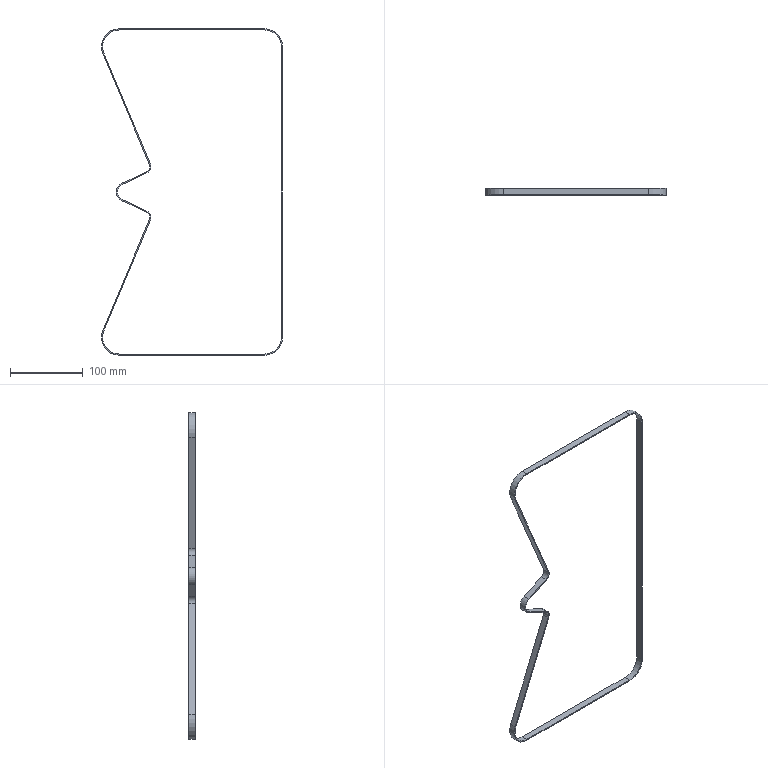Part | SolidWorks | features Extrusion 1 | 1 solid | 30 faces | box 248.84 x 9 x 448.84 mm | volume 19272 mm3 | plane 16 | cylinder 14 | commonest cylinder face diameters 45.84 x4 48.84 x4 16 x2 19 x2 22.92 x1 25.92 x1
STEP:
#1=CARTESIAN_POINT('',(121.194,9.,924.42));
#2=VERTEX_POINT('',#1);
#3=CARTESIAN_POINT('',(145.614,9.,900.));
#4=VERTEX_POINT('',#3);
#5=CARTESIAN_POINT('',(121.194,9.,900.));
#6=DIRECTION('',(0.,1.,0.));
#7=DIRECTION('',(0.,0.,1.));
#8=AXIS2_PLACEMENT_3D('',#5,#6,#7);
#9=CIRCLE('',#8,24.42);
#10=EDGE_CURVE('',#2,#4,#9,.T.);
#11=ORIENTED_EDGE('',*,*,#10,.T.);
#12=CARTESIAN_POINT('',(145.614,9.,500.));
#13=VERTEX_POINT('',#12);
#14=CARTESIAN_POINT('',(145.614,9.,900.));
#15=DIRECTION('',(0.,0.,-1.));
#16=VECTOR('',#15,1000.);
#17=LINE('',#14,#16);
#18=EDGE_CURVE('',#4,#13,#17,.T.);
#19=ORIENTED_EDGE('',*,*,#18,.T.);
#20=CARTESIAN_POINT('',(121.194,9.,475.58));
#21=VERTEX_POINT('',#20);
#22=CARTESIAN_POINT('',(121.194,9.,500.));
#23=DIRECTION('',(0.,1.,0.));
#24=DIRECTION('',(0.,0.,1.));
#25=AXIS2_PLACEMENT_3D('',#22,#23,#24);
#26=CIRCLE('',#25,24.42);
#27=EDGE_CURVE('',#13,#21,#26,.T.);
#28=ORIENTED_EDGE('',*,*,#27,.T.);
#29=CARTESIAN_POINT('',(-78.806,9.,475.58));
#30=VERTEX_POINT('',#29);
#31=CARTESIAN_POINT('',(121.194,9.,475.58));
#32=DIRECTION('',(-1.,0.,0.));
#33=VECTOR('',#32,1000.);
#34=LINE('',#31,#33);
#35=EDGE_CURVE('',#21,#30,#34,.T.);
#36=ORIENTED_EDGE('',*,*,#35,.T.);
#37=CARTESIAN_POINT('',(-101.328,9.,509.439));
#38=VERTEX_POINT('',#37);
#39=CARTESIAN_POINT('',(-78.806,9.,500.));
#40=DIRECTION('',(0.,1.,0.));
#41=DIRECTION('',(0.,0.,1.));
#42=AXIS2_PLACEMENT_3D('',#39,#40,#41);
#43=CIRCLE('',#42,24.42);
#44=EDGE_CURVE('',#30,#38,#43,.T.);
#45=ORIENTED_EDGE('',*,*,#44,.T.);
#46=CARTESIAN_POINT('',(-37.428,9.,661.908));
#47=VERTEX_POINT('',#46);
#48=CARTESIAN_POINT('',(-37.428,9.,661.908));
#49=DIRECTION('',(0.3865,0.,0.9223));
#50=VECTOR('',#49,1000.);
#51=LINE('',#48,#50);
#52=EDGE_CURVE('',#38,#47,#51,.T.);
#53=ORIENTED_EDGE('',*,*,#52,.T.);
#54=CARTESIAN_POINT('',(-41.387,9.,672.233));
#55=VERTEX_POINT('',#54);
#56=CARTESIAN_POINT('',(-44.806,9.,665.));
#57=DIRECTION('',(0.,-1.,0.));
#58=DIRECTION('',(0.,0.,1.));
#59=AXIS2_PLACEMENT_3D('',#56,#57,#58);
#60=CIRCLE('',#59,8.);
#61=EDGE_CURVE('',#47,#55,#60,.T.);
#62=ORIENTED_EDGE('',*,*,#61,.T.);
#63=CARTESIAN_POINT('',(-75.344,9.,688.283));
#64=VERTEX_POINT('',#63);
#65=CARTESIAN_POINT('',(-75.344,9.,688.283));
#66=DIRECTION('',(-0.9041,0.,0.4273));
#67=VECTOR('',#66,1000.);
#68=LINE('',#65,#67);
#69=EDGE_CURVE('',#55,#64,#68,.T.);
#70=ORIENTED_EDGE('',*,*,#69,.T.);
#71=CARTESIAN_POINT('',(-75.344,9.,711.717));
#72=VERTEX_POINT('',#71);
#73=CARTESIAN_POINT('',(-69.806,9.,700.));
#74=DIRECTION('',(0.,1.,0.));
#75=DIRECTION('',(0.,0.,1.));
#76=AXIS2_PLACEMENT_3D('',#73,#74,#75);
#77=CIRCLE('',#76,12.96);
#78=EDGE_CURVE('',#64,#72,#77,.T.);
#79=ORIENTED_EDGE('',*,*,#78,.T.);
#80=CARTESIAN_POINT('',(-41.387,9.,727.767));
#81=VERTEX_POINT('',#80);
#82=CARTESIAN_POINT('',(-75.344,9.,711.717));
#83=DIRECTION('',(0.9041,0.,0.4273));
#84=VECTOR('',#83,1000.);
#85=LINE('',#82,#84);
#86=EDGE_CURVE('',#72,#81,#85,.T.);
#87=ORIENTED_EDGE('',*,*,#86,.T.);
#88=CARTESIAN_POINT('',(-37.428,9.,738.092));
#89=VERTEX_POINT('',#88);
#90=CARTESIAN_POINT('',(-44.806,9.,735.));
#91=DIRECTION('',(0.,-1.,0.));
#92=DIRECTION('',(0.,0.,1.));
#93=AXIS2_PLACEMENT_3D('',#90,#91,#92);
#94=CIRCLE('',#93,8.);
#95=EDGE_CURVE('',#81,#89,#94,.T.);
#96=ORIENTED_EDGE('',*,*,#95,.T.);
#97=CARTESIAN_POINT('',(-101.328,9.,890.561));
#98=VERTEX_POINT('',#97);
#99=CARTESIAN_POINT('',(-37.428,9.,738.092));
#100=DIRECTION('',(-0.3865,0.,0.9223));
#101=VECTOR('',#100,1000.);
#102=LINE('',#99,#101);
#103=EDGE_CURVE('',#89,#98,#102,.T.);
#104=ORIENTED_EDGE('',*,*,#103,.T.);
#105=CARTESIAN_POINT('',(-78.806,9.,924.42));
#106=VERTEX_POINT('',#105);
#107=CARTESIAN_POINT('',(-78.806,9.,900.));
#108=DIRECTION('',(0.,1.,0.));
#109=DIRECTION('',(0.,0.,1.));
#110=AXIS2_PLACEMENT_3D('',#107,#108,#109);
#111=CIRCLE('',#110,24.42);
#112=EDGE_CURVE('',#98,#106,#111,.T.);
#113=ORIENTED_EDGE('',*,*,#112,.T.);
#114=CARTESIAN_POINT('',(121.194,9.,924.42));
#115=DIRECTION('',(1.,0.,0.));
#116=VECTOR('',#115,1000.);
#117=LINE('',#114,#116);
#118=EDGE_CURVE('',#106,#2,#117,.T.);
#119=ORIENTED_EDGE('',*,*,#118,.T.);
#120=EDGE_LOOP('',(#11,#19,#28,#36,#45,#53,#62,#70,#79,#87,#96,#104,#113,#119));
#121=FACE_OUTER_BOUND('',#120,.T.);
#122=CARTESIAN_POINT('',(-40.746,9.,673.589));
#123=VERTEX_POINT('',#122);
#124=CARTESIAN_POINT('',(-74.703,9.,689.639));
#125=VERTEX_POINT('',#124);
#126=CARTESIAN_POINT('',(-74.703,9.,689.639));
#127=DIRECTION('',(-0.9041,0.,0.4273));
#128=VECTOR('',#127,1000.);
#129=LINE('',#126,#128);
#130=EDGE_CURVE('',#123,#125,#129,.T.);
#131=ORIENTED_EDGE('',*,*,#130,.F.);
#132=CARTESIAN_POINT('',(-36.044,9.,661.328));
#133=VERTEX_POINT('',#132);
#134=CARTESIAN_POINT('',(-44.806,9.,665.));
#135=DIRECTION('',(0.,-1.,0.));
#136=DIRECTION('',(0.,0.,1.));
#137=AXIS2_PLACEMENT_3D('',#134,#135,#136);
#138=CIRCLE('',#137,9.5);
#139=EDGE_CURVE('',#133,#123,#138,.T.);
#140=ORIENTED_EDGE('',*,*,#139,.F.);
#141=CARTESIAN_POINT('',(-99.945,9.,508.859));
#142=VERTEX_POINT('',#141);
#143=CARTESIAN_POINT('',(-36.044,9.,661.328));
#144=DIRECTION('',(0.3865,0.,0.9223));
#145=VECTOR('',#144,1000.);
#146=LINE('',#143,#145);
#147=EDGE_CURVE('',#142,#133,#146,.T.);
#148=ORIENTED_EDGE('',*,*,#147,.F.);
#149=CARTESIAN_POINT('',(-78.806,9.,477.08));
#150=VERTEX_POINT('',#149);
#151=CARTESIAN_POINT('',(-78.806,9.,500.));
#152=DIRECTION('',(0.,1.,0.));
#153=DIRECTION('',(0.,0.,1.));
#154=AXIS2_PLACEMENT_3D('',#151,#152,#153);
#155=CIRCLE('',#154,22.92);
#156=EDGE_CURVE('',#150,#142,#155,.T.);
#157=ORIENTED_EDGE('',*,*,#156,.F.);
#158=CARTESIAN_POINT('',(121.194,9.,477.08));
#159=VERTEX_POINT('',#158);
#160=CARTESIAN_POINT('',(121.194,9.,477.08));
#161=DIRECTION('',(-1.,0.,0.));
#162=VECTOR('',#161,1000.);
#163=LINE('',#160,#162);
#164=EDGE_CURVE('',#159,#150,#163,.T.);
#165=ORIENTED_EDGE('',*,*,#164,.F.);
#166=CARTESIAN_POINT('',(144.114,9.,500.));
#167=VERTEX_POINT('',#166);
#168=CARTESIAN_POINT('',(121.194,9.,500.));
#169=DIRECTION('',(0.,1.,0.));
#170=DIRECTION('',(0.,0.,1.));
#171=AXIS2_PLACEMENT_3D('',#168,#169,#170);
#172=CIRCLE('',#171,22.92);
#173=EDGE_CURVE('',#167,#159,#172,.T.);
#174=ORIENTED_EDGE('',*,*,#173,.F.);
#175=CARTESIAN_POINT('',(144.114,9.,900.));
#176=VERTEX_POINT('',#175);
#177=CARTESIAN_POINT('',(144.114,9.,900.));
#178=DIRECTION('',(0.,0.,-1.));
#179=VECTOR('',#178,1000.);
#180=LINE('',#177,#179);
#181=EDGE_CURVE('',#176,#167,#180,.T.);
#182=ORIENTED_EDGE('',*,*,#181,.F.);
#183=CARTESIAN_POINT('',(121.194,9.,922.92));
#184=VERTEX_POINT('',#183);
#185=CARTESIAN_POINT('',(121.194,9.,900.));
#186=DIRECTION('',(0.,1.,0.));
#187=DIRECTION('',(0.,0.,1.));
#188=AXIS2_PLACEMENT_3D('',#185,#186,#187);
#189=CIRCLE('',#188,22.92);
#190=EDGE_CURVE('',#184,#176,#189,.T.);
#191=ORIENTED_EDGE('',*,*,#190,.F.);
#192=CARTESIAN_POINT('',(-78.806,9.,922.92));
#193=VERTEX_POINT('',#192);
#194=CARTESIAN_POINT('',(121.194,9.,922.92));
#195=DIRECTION('',(1.,0.,0.));
#196=VECTOR('',#195,1000.);
#197=LINE('',#194,#196);
#198=EDGE_CURVE('',#193,#184,#197,.T.);
#199=ORIENTED_EDGE('',*,*,#198,.F.);
#200=CARTESIAN_POINT('',(-99.945,9.,891.141));
#201=VERTEX_POINT('',#200);
#202=CARTESIAN_POINT('',(-78.806,9.,900.));
#203=DIRECTION('',(0.,1.,0.));
#204=DIRECTION('',(0.,0.,1.));
#205=AXIS2_PLACEMENT_3D('',#202,#203,#204);
#206=CIRCLE('',#205,22.92);
#207=EDGE_CURVE('',#201,#193,#206,.T.);
#208=ORIENTED_EDGE('',*,*,#207,.F.);
#209=CARTESIAN_POINT('',(-36.044,9.,738.672));
#210=VERTEX_POINT('',#209);
#211=CARTESIAN_POINT('',(-36.044,9.,738.672));
#212=DIRECTION('',(-0.3865,0.,0.9223));
#213=VECTOR('',#212,1000.);
#214=LINE('',#211,#213);
#215=EDGE_CURVE('',#210,#201,#214,.T.);
#216=ORIENTED_EDGE('',*,*,#215,.F.);
#217=CARTESIAN_POINT('',(-40.746,9.,726.411));
#218=VERTEX_POINT('',#217);
#219=CARTESIAN_POINT('',(-44.806,9.,735.));
#220=DIRECTION('',(0.,-1.,0.));
#221=DIRECTION('',(0.,0.,1.));
#222=AXIS2_PLACEMENT_3D('',#219,#220,#221);
#223=CIRCLE('',#222,9.5);
#224=EDGE_CURVE('',#218,#210,#223,.T.);
#225=ORIENTED_EDGE('',*,*,#224,.F.);
#226=CARTESIAN_POINT('',(-74.703,9.,710.361));
#227=VERTEX_POINT('',#226);
#228=CARTESIAN_POINT('',(-74.703,9.,710.361));
#229=DIRECTION('',(0.9041,0.,0.4273));
#230=VECTOR('',#229,1000.);
#231=LINE('',#228,#230);
#232=EDGE_CURVE('',#227,#218,#231,.T.);
#233=ORIENTED_EDGE('',*,*,#232,.F.);
#234=CARTESIAN_POINT('',(-69.806,9.,700.));
#235=DIRECTION('',(0.,1.,0.));
#236=DIRECTION('',(0.,0.,1.));
#237=AXIS2_PLACEMENT_3D('',#234,#235,#236);
#238=CIRCLE('',#237,11.46);
#239=EDGE_CURVE('',#125,#227,#238,.T.);
#240=ORIENTED_EDGE('',*,*,#239,.F.);
#241=EDGE_LOOP('',(#131,#140,#148,#157,#165,#174,#182,#191,#199,#208,#216,#225,#233,#240));
#242=FACE_BOUND('',#241,.T.);
#243=CARTESIAN_POINT('',(121.194,9.,900.));
#244=DIRECTION('',(0.,1.,0.));
#245=DIRECTION('',(0.,0.,1.));
#246=AXIS2_PLACEMENT_3D('',#243,#244,#245);
#247=PLANE('',#246);
#248=ADVANCED_FACE('',(#121,#242),#247,.T.);
#249=CARTESIAN_POINT('',(121.194,0.,924.42));
#250=VERTEX_POINT('',#249);
#251=CARTESIAN_POINT('',(145.614,0.,900.));
#252=VERTEX_POINT('',#251);
#253=CARTESIAN_POINT('',(121.194,0.,900.));
#254=DIRECTION('',(0.,1.,0.));
#255=DIRECTION('',(0.,0.,1.));
#256=AXIS2_PLACEMENT_3D('',#253,#254,#255);
#257=CIRCLE('',#256,24.42);
#258=EDGE_CURVE('',#250,#252,#257,.T.);
#259=ORIENTED_EDGE('',*,*,#258,.F.);
#260=CARTESIAN_POINT('',(-78.806,0.,924.42));
#261=VERTEX_POINT('',#260);
#262=CARTESIAN_POINT('',(121.194,0.,924.42));
#263=DIRECTION('',(1.,0.,0.));
#264=VECTOR('',#263,1000.);
#265=LINE('',#262,#264);
#266=EDGE_CURVE('',#261,#250,#265,.T.);
#267=ORIENTED_EDGE('',*,*,#266,.F.);
#268=CARTESIAN_POINT('',(-101.328,0.,890.561));
#269=VERTEX_POINT('',#268);
#270=CARTESIAN_POINT('',(-78.806,0.,900.));
#271=DIRECTION('',(0.,1.,0.));
#272=DIRECTION('',(0.,0.,1.));
#273=AXIS2_PLACEMENT_3D('',#270,#271,#272);
#274=CIRCLE('',#273,24.42);
#275=EDGE_CURVE('',#269,#261,#274,.T.);
#276=ORIENTED_EDGE('',*,*,#275,.F.);
#277=CARTESIAN_POINT('',(-37.428,0.,738.092));
#278=VERTEX_POINT('',#277);
#279=CARTESIAN_POINT('',(-37.428,0.,738.092));
#280=DIRECTION('',(-0.3865,0.,0.9223));
#281=VECTOR('',#280,1000.);
#282=LINE('',#279,#281);
#283=EDGE_CURVE('',#278,#269,#282,.T.);
#284=ORIENTED_EDGE('',*,*,#283,.F.);
#285=CARTESIAN_POINT('',(-41.387,0.,727.767));
#286=VERTEX_POINT('',#285);
#287=CARTESIAN_POINT('',(-44.806,0.,735.));
#288=DIRECTION('',(0.,-1.,0.));
#289=DIRECTION('',(0.,0.,1.));
#290=AXIS2_PLACEMENT_3D('',#287,#288,#289);
#291=CIRCLE('',#290,8.);
#292=EDGE_CURVE('',#286,#278,#291,.T.);
#293=ORIENTED_EDGE('',*,*,#292,.F.);
#294=CARTESIAN_POINT('',(-75.344,0.,711.717));
#295=VERTEX_POINT('',#294);
#296=CARTESIAN_POINT('',(-75.344,0.,711.717));
#297=DIRECTION('',(0.9041,0.,0.4273));
#298=VECTOR('',#297,1000.);
#299=LINE('',#296,#298);
#300=EDGE_CURVE('',#295,#286,#299,.T.);
#301=ORIENTED_EDGE('',*,*,#300,.F.);
#302=CARTESIAN_POINT('',(-75.344,0.,688.283));
#303=VERTEX_POINT('',#302);
#304=CARTESIAN_POINT('',(-69.806,0.,700.));
#305=DIRECTION('',(0.,1.,0.));
#306=DIRECTION('',(0.,0.,1.));
#307=AXIS2_PLACEMENT_3D('',#304,#305,#306);
#308=CIRCLE('',#307,12.96);
#309=EDGE_CURVE('',#303,#295,#308,.T.);
#310=ORIENTED_EDGE('',*,*,#309,.F.);
#311=CARTESIAN_POINT('',(-41.387,0.,672.233));
#312=VERTEX_POINT('',#311);
#313=CARTESIAN_POINT('',(-75.344,0.,688.283));
#314=DIRECTION('',(-0.9041,0.,0.4273));
#315=VECTOR('',#314,1000.);
#316=LINE('',#313,#315);
#317=EDGE_CURVE('',#312,#303,#316,.T.);
#318=ORIENTED_EDGE('',*,*,#317,.F.);
#319=CARTESIAN_POINT('',(-37.428,0.,661.908));
#320=VERTEX_POINT('',#319);
#321=CARTESIAN_POINT('',(-44.806,0.,665.));
#322=DIRECTION('',(0.,-1.,0.));
#323=DIRECTION('',(0.,0.,1.));
#324=AXIS2_PLACEMENT_3D('',#321,#322,#323);
#325=CIRCLE('',#324,8.);
#326=EDGE_CURVE('',#320,#312,#325,.T.);
#327=ORIENTED_EDGE('',*,*,#326,.F.);
#328=CARTESIAN_POINT('',(-101.328,0.,509.439));
#329=VERTEX_POINT('',#328);
#330=CARTESIAN_POINT('',(-37.428,0.,661.908));
#331=DIRECTION('',(0.3865,0.,0.9223));
#332=VECTOR('',#331,1000.);
#333=LINE('',#330,#332);
#334=EDGE_CURVE('',#329,#320,#333,.T.);
#335=ORIENTED_EDGE('',*,*,#334,.F.);
#336=CARTESIAN_POINT('',(-78.806,0.,475.58));
#337=VERTEX_POINT('',#336);
#338=CARTESIAN_POINT('',(-78.806,0.,500.));
#339=DIRECTION('',(0.,1.,0.));
#340=DIRECTION('',(0.,0.,1.));
#341=AXIS2_PLACEMENT_3D('',#338,#339,#340);
#342=CIRCLE('',#341,24.42);
#343=EDGE_CURVE('',#337,#329,#342,.T.);
#344=ORIENTED_EDGE('',*,*,#343,.F.);
#345=CARTESIAN_POINT('',(121.194,0.,475.58));
#346=VERTEX_POINT('',#345);
#347=CARTESIAN_POINT('',(121.194,0.,475.58));
#348=DIRECTION('',(-1.,0.,0.));
#349=VECTOR('',#348,1000.);
#350=LINE('',#347,#349);
#351=EDGE_CURVE('',#346,#337,#350,.T.);
#352=ORIENTED_EDGE('',*,*,#351,.F.);
#353=CARTESIAN_POINT('',(145.614,0.,500.));
#354=VERTEX_POINT('',#353);
#355=CARTESIAN_POINT('',(121.194,0.,500.));
#356=DIRECTION('',(0.,1.,0.));
#357=DIRECTION('',(0.,0.,1.));
#358=AXIS2_PLACEMENT_3D('',#355,#356,#357);
#359=CIRCLE('',#358,24.42);
#360=EDGE_CURVE('',#354,#346,#359,.T.);
#361=ORIENTED_EDGE('',*,*,#360,.F.);
#362=CARTESIAN_POINT('',(145.614,0.,900.));
#363=DIRECTION('',(0.,0.,-1.));
#364=VECTOR('',#363,1000.);
#365=LINE('',#362,#364);
#366=EDGE_CURVE('',#252,#354,#365,.T.);
#367=ORIENTED_EDGE('',*,*,#366,.F.);
#368=EDGE_LOOP('',(#259,#267,#276,#284,#293,#301,#310,#318,#327,#335,#344,#352,#361,#367));
#369=FACE_OUTER_BOUND('',#368,.T.);
#370=CARTESIAN_POINT('',(-36.044,0.,661.328));
#371=VERTEX_POINT('',#370);
#372=CARTESIAN_POINT('',(-40.746,0.,673.589));
#373=VERTEX_POINT('',#372);
#374=CARTESIAN_POINT('',(-44.806,0.,665.));
#375=DIRECTION('',(0.,-1.,0.));
#376=DIRECTION('',(0.,0.,1.));
#377=AXIS2_PLACEMENT_3D('',#374,#375,#376);
#378=CIRCLE('',#377,9.5);
#379=EDGE_CURVE('',#371,#373,#378,.T.);
#380=ORIENTED_EDGE('',*,*,#379,.T.);
#381=CARTESIAN_POINT('',(-74.703,0.,689.639));
#382=VERTEX_POINT('',#381);
#383=CARTESIAN_POINT('',(-74.703,0.,689.639));
#384=DIRECTION('',(-0.9041,0.,0.4273));
#385=VECTOR('',#384,1000.);
#386=LINE('',#383,#385);
#387=EDGE_CURVE('',#373,#382,#386,.T.);
#388=ORIENTED_EDGE('',*,*,#387,.T.);
#389=CARTESIAN_POINT('',(-74.703,0.,710.361));
#390=VERTEX_POINT('',#389);
#391=CARTESIAN_POINT('',(-69.806,0.,700.));
#392=DIRECTION('',(0.,1.,0.));
#393=DIRECTION('',(0.,0.,1.));
#394=AXIS2_PLACEMENT_3D('',#391,#392,#393);
#395=CIRCLE('',#394,11.46);
#396=EDGE_CURVE('',#382,#390,#395,.T.);
#397=ORIENTED_EDGE('',*,*,#396,.T.);
#398=CARTESIAN_POINT('',(-40.746,0.,726.411));
#399=VERTEX_POINT('',#398);
#400=CARTESIAN_POINT('',(-74.703,0.,710.361));
#401=DIRECTION('',(0.9041,0.,0.4273));
#402=VECTOR('',#401,1000.);
#403=LINE('',#400,#402);
#404=EDGE_CURVE('',#390,#399,#403,.T.);
#405=ORIENTED_EDGE('',*,*,#404,.T.);
#406=CARTESIAN_POINT('',(-36.044,0.,738.672));
#407=VERTEX_POINT('',#406);
#408=CARTESIAN_POINT('',(-44.806,0.,735.));
#409=DIRECTION('',(0.,-1.,0.));
#410=DIRECTION('',(0.,0.,1.));
#411=AXIS2_PLACEMENT_3D('',#408,#409,#410);
#412=CIRCLE('',#411,9.5);
#413=EDGE_CURVE('',#399,#407,#412,.T.);
#414=ORIENTED_EDGE('',*,*,#413,.T.);
#415=CARTESIAN_POINT('',(-99.945,0.,891.141));
#416=VERTEX_POINT('',#415);
#417=CARTESIAN_POINT('',(-36.044,0.,738.672));
#418=DIRECTION('',(-0.3865,0.,0.9223));
#419=VECTOR('',#418,1000.);
#420=LINE('',#417,#419);
#421=EDGE_CURVE('',#407,#416,#420,.T.);
#422=ORIENTED_EDGE('',*,*,#421,.T.);
#423=CARTESIAN_POINT('',(-78.806,0.,922.92));
#424=VERTEX_POINT('',#423);
#425=CARTESIAN_POINT('',(-78.806,0.,900.));
#426=DIRECTION('',(0.,1.,0.));
#427=DIRECTION('',(0.,0.,1.));
#428=AXIS2_PLACEMENT_3D('',#425,#426,#427);
#429=CIRCLE('',#428,22.92);
#430=EDGE_CURVE('',#416,#424,#429,.T.);
#431=ORIENTED_EDGE('',*,*,#430,.T.);
#432=CARTESIAN_POINT('',(121.194,0.,922.92));
#433=VERTEX_POINT('',#432);
#434=CARTESIAN_POINT('',(121.194,0.,922.92));
#435=DIRECTION('',(1.,0.,0.));
#436=VECTOR('',#435,1000.);
#437=LINE('',#434,#436);
#438=EDGE_CURVE('',#424,#433,#437,.T.);
#439=ORIENTED_EDGE('',*,*,#438,.T.);
#440=CARTESIAN_POINT('',(144.114,0.,900.));
#441=VERTEX_POINT('',#440);
#442=CARTESIAN_POINT('',(121.194,0.,900.));
#443=DIRECTION('',(0.,1.,0.));
#444=DIRECTION('',(0.,0.,1.));
#445=AXIS2_PLACEMENT_3D('',#442,#443,#444);
#446=CIRCLE('',#445,22.92);
#447=EDGE_CURVE('',#433,#441,#446,.T.);
#448=ORIENTED_EDGE('',*,*,#447,.T.);
#449=CARTESIAN_POINT('',(144.114,0.,500.));
#450=VERTEX_POINT('',#449);
#451=CARTESIAN_POINT('',(144.114,0.,900.));
#452=DIRECTION('',(0.,0.,-1.));
#453=VECTOR('',#452,1000.);
#454=LINE('',#451,#453);
#455=EDGE_CURVE('',#441,#450,#454,.T.);
#456=ORIENTED_EDGE('',*,*,#455,.T.);
#457=CARTESIAN_POINT('',(121.194,0.,477.08));
#458=VERTEX_POINT('',#457);
#459=CARTESIAN_POINT('',(121.194,0.,500.));
#460=DIRECTION('',(0.,1.,0.));
#461=DIRECTION('',(0.,0.,1.));
#462=AXIS2_PLACEMENT_3D('',#459,#460,#461);
#463=CIRCLE('',#462,22.92);
#464=EDGE_CURVE('',#450,#458,#463,.T.);
#465=ORIENTED_EDGE('',*,*,#464,.T.);
#466=CARTESIAN_POINT('',(-78.806,0.,477.08));
#467=VERTEX_POINT('',#466);
#468=CARTESIAN_POINT('',(121.194,0.,477.08));
#469=DIRECTION('',(-1.,0.,0.));
#470=VECTOR('',#469,1000.);
#471=LINE('',#468,#470);
#472=EDGE_CURVE('',#458,#467,#471,.T.);
#473=ORIENTED_EDGE('',*,*,#472,.T.);
#474=CARTESIAN_POINT('',(-99.945,0.,508.859));
#475=VERTEX_POINT('',#474);
#476=CARTESIAN_POINT('',(-78.806,0.,500.));
#477=DIRECTION('',(0.,1.,0.));
#478=DIRECTION('',(0.,0.,1.));
#479=AXIS2_PLACEMENT_3D('',#476,#477,#478);
#480=CIRCLE('',#479,22.92);
#481=EDGE_CURVE('',#467,#475,#480,.T.);
#482=ORIENTED_EDGE('',*,*,#481,.T.);
#483=CARTESIAN_POINT('',(-36.044,0.,661.328));
#484=DIRECTION('',(0.3865,0.,0.9223));
#485=VECTOR('',#484,1000.);
#486=LINE('',#483,#485);
#487=EDGE_CURVE('',#475,#371,#486,.T.);
#488=ORIENTED_EDGE('',*,*,#487,.T.);
#489=EDGE_LOOP('',(#380,#388,#397,#405,#414,#422,#431,#439,#448,#456,#465,#473,#482,#488));
#490=FACE_BOUND('',#489,.T.);
#491=CARTESIAN_POINT('',(121.194,0.,900.));
#492=DIRECTION('',(0.,1.,0.));
#493=DIRECTION('',(0.,0.,1.));
#494=AXIS2_PLACEMENT_3D('',#491,#492,#493);
#495=PLANE('',#494);
#496=ADVANCED_FACE('',(#369,#490),#495,.F.);
#497=ORIENTED_EDGE('',*,*,#258,.T.);
#498=CARTESIAN_POINT('',(145.614,9.,900.));
#499=DIRECTION('',(0.,-1.,0.));
#500=VECTOR('',#499,1000.);
#501=LINE('',#498,#500);
#502=EDGE_CURVE('',#4,#252,#501,.T.);
#503=ORIENTED_EDGE('',*,*,#502,.F.);
#504=ORIENTED_EDGE('',*,*,#10,.F.);
#505=CARTESIAN_POINT('',(121.194,9.,924.42));
#506=DIRECTION('',(0.,-1.,0.));
#507=VECTOR('',#506,1000.);
#508=LINE('',#505,#507);
#509=EDGE_CURVE('',#2,#250,#508,.T.);
#510=ORIENTED_EDGE('',*,*,#509,.T.);
#511=EDGE_LOOP('',(#497,#503,#504,#510));
#512=FACE_OUTER_BOUND('',#511,.T.);
#513=CARTESIAN_POINT('',(121.194,9.,900.));
#514=DIRECTION('',(0.,-1.,0.));
#515=DIRECTION('',(0.,0.,-1.));
#516=AXIS2_PLACEMENT_3D('',#513,#514,#515);
#517=CYLINDRICAL_SURFACE('',#516,24.42);
#518=ADVANCED_FACE('',(#512),#517,.T.);
#519=ORIENTED_EDGE('',*,*,#366,.T.);
#520=CARTESIAN_POINT('',(145.614,9.,500.));
#521=DIRECTION('',(0.,-1.,0.));
#522=VECTOR('',#521,1000.);
#523=LINE('',#520,#522);
#524=EDGE_CURVE('',#13,#354,#523,.T.);
#525=ORIENTED_EDGE('',*,*,#524,.F.);
#526=ORIENTED_EDGE('',*,*,#18,.F.);
#527=ORIENTED_EDGE('',*,*,#502,.T.);
#528=EDGE_LOOP('',(#519,#525,#526,#527));
#529=FACE_OUTER_BOUND('',#528,.T.);
#530=CARTESIAN_POINT('',(145.614,9.,900.));
#531=DIRECTION('',(-1.,0.,0.));
#532=DIRECTION('',(0.,0.,1.));
#533=AXIS2_PLACEMENT_3D('',#530,#531,#532);
#534=PLANE('',#533);
#535=ADVANCED_FACE('',(#529),#534,.F.);
#536=ORIENTED_EDGE('',*,*,#360,.T.);
#537=CARTESIAN_POINT('',(121.194,9.,475.58));
#538=DIRECTION('',(0.,-1.,0.));
#539=VECTOR('',#538,1000.);
#540=LINE('',#537,#539);
#541=EDGE_CURVE('',#21,#346,#540,.T.);
#542=ORIENTED_EDGE('',*,*,#541,.F.);
#543=ORIENTED_EDGE('',*,*,#27,.F.);
#544=ORIENTED_EDGE('',*,*,#524,.T.);
#545=EDGE_LOOP('',(#536,#542,#543,#544));
#546=FACE_OUTER_BOUND('',#545,.T.);
#547=CARTESIAN_POINT('',(121.194,9.,500.));
#548=DIRECTION('',(0.,-1.,0.));
#549=DIRECTION('',(0.,0.,-1.));
#550=AXIS2_PLACEMENT_3D('',#547,#548,#549);
#551=CYLINDRICAL_SURFACE('',#550,24.42);
#552=ADVANCED_FACE('',(#546),#551,.T.);
#553=ORIENTED_EDGE('',*,*,#351,.T.);
#554=CARTESIAN_POINT('',(-78.806,9.,475.58));
#555=DIRECTION('',(0.,-1.,0.));
#556=VECTOR('',#555,1000.);
#557=LINE('',#554,#556);
#558=EDGE_CURVE('',#30,#337,#557,.T.);
#559=ORIENTED_EDGE('',*,*,#558,.F.);
#560=ORIENTED_EDGE('',*,*,#35,.F.);
#561=ORIENTED_EDGE('',*,*,#541,.T.);
#562=EDGE_LOOP('',(#553,#559,#560,#561));
#563=FACE_OUTER_BOUND('',#562,.T.);
#564=CARTESIAN_POINT('',(121.194,9.,475.58));
#565=DIRECTION('',(0.,0.,1.));
#566=DIRECTION('',(1.,0.,0.));
#567=AXIS2_PLACEMENT_3D('',#564,#565,#566);
#568=PLANE('',#567);
#569=ADVANCED_FACE('',(#563),#568,.F.);
#570=ORIENTED_EDGE('',*,*,#343,.T.);
#571=CARTESIAN_POINT('',(-101.328,9.,509.439));
#572=DIRECTION('',(0.,-1.,0.));
#573=VECTOR('',#572,1000.);
#574=LINE('',#571,#573);
#575=EDGE_CURVE('',#38,#329,#574,.T.);
#576=ORIENTED_EDGE('',*,*,#575,.F.);
#577=ORIENTED_EDGE('',*,*,#44,.F.);
#578=ORIENTED_EDGE('',*,*,#558,.T.);
#579=EDGE_LOOP('',(#570,#576,#577,#578));
#580=FACE_OUTER_BOUND('',#579,.T.);
#581=CARTESIAN_POINT('',(-78.806,9.,500.));
#582=DIRECTION('',(0.,-1.,0.));
#583=DIRECTION('',(0.,0.,-1.));
#584=AXIS2_PLACEMENT_3D('',#581,#582,#583);
#585=CYLINDRICAL_SURFACE('',#584,24.42);
#586=ADVANCED_FACE('',(#580),#585,.T.);
#587=ORIENTED_EDGE('',*,*,#334,.T.);
#588=CARTESIAN_POINT('',(-37.428,9.,661.908));
#589=DIRECTION('',(0.,-1.,0.));
#590=VECTOR('',#589,1000.);
#591=LINE('',#588,#590);
#592=EDGE_CURVE('',#47,#320,#591,.T.);
#593=ORIENTED_EDGE('',*,*,#592,.F.);
#594=ORIENTED_EDGE('',*,*,#52,.F.);
#595=ORIENTED_EDGE('',*,*,#575,.T.);
#596=EDGE_LOOP('',(#587,#593,#594,#595));
#597=FACE_OUTER_BOUND('',#596,.T.);
#598=CARTESIAN_POINT('',(-37.428,9.,661.908));
#599=DIRECTION('',(0.9223,0.,-0.3865));
#600=DIRECTION('',(-0.3865,0.,-0.9223));
#601=AXIS2_PLACEMENT_3D('',#598,#599,#600);
#602=PLANE('',#601);
#603=ADVANCED_FACE('',(#597),#602,.F.);
#604=ORIENTED_EDGE('',*,*,#326,.T.);
#605=CARTESIAN_POINT('',(-41.387,9.,672.233));
#606=DIRECTION('',(0.,-1.,0.));
#607=VECTOR('',#606,1000.);
#608=LINE('',#605,#607);
#609=EDGE_CURVE('',#55,#312,#608,.T.);
#610=ORIENTED_EDGE('',*,*,#609,.F.);
#611=ORIENTED_EDGE('',*,*,#61,.F.);
#612=ORIENTED_EDGE('',*,*,#592,.T.);
#613=EDGE_LOOP('',(#604,#610,#611,#612));
#614=FACE_OUTER_BOUND('',#613,.T.);
#615=CARTESIAN_POINT('',(-44.806,9.,665.));
#616=DIRECTION('',(0.,-1.,0.));
#617=DIRECTION('',(0.,0.,-1.));
#618=AXIS2_PLACEMENT_3D('',#615,#616,#617);
#619=CYLINDRICAL_SURFACE('',#618,8.);
#620=ADVANCED_FACE('',(#614),#619,.F.);
#621=ORIENTED_EDGE('',*,*,#317,.T.);
#622=CARTESIAN_POINT('',(-75.344,9.,688.283));
#623=DIRECTION('',(0.,-1.,0.));
#624=VECTOR('',#623,1000.);
#625=LINE('',#622,#624);
#626=EDGE_CURVE('',#64,#303,#625,.T.);
#627=ORIENTED_EDGE('',*,*,#626,.F.);
#628=ORIENTED_EDGE('',*,*,#69,.F.);
#629=ORIENTED_EDGE('',*,*,#609,.T.);
#630=EDGE_LOOP('',(#621,#627,#628,#629));
#631=FACE_OUTER_BOUND('',#630,.T.);
#632=CARTESIAN_POINT('',(-75.344,9.,688.283));
#633=DIRECTION('',(0.4273,0.,0.9041));
#634=DIRECTION('',(0.9041,0.,-0.4273));
#635=AXIS2_PLACEMENT_3D('',#632,#633,#634);
#636=PLANE('',#635);
#637=ADVANCED_FACE('',(#631),#636,.F.);
#638=ORIENTED_EDGE('',*,*,#309,.T.);
#639=CARTESIAN_POINT('',(-75.344,9.,711.717));
#640=DIRECTION('',(0.,-1.,0.));
#641=VECTOR('',#640,1000.);
#642=LINE('',#639,#641);
#643=EDGE_CURVE('',#72,#295,#642,.T.);
#644=ORIENTED_EDGE('',*,*,#643,.F.);
#645=ORIENTED_EDGE('',*,*,#78,.F.);
#646=ORIENTED_EDGE('',*,*,#626,.T.);
#647=EDGE_LOOP('',(#638,#644,#645,#646));
#648=FACE_OUTER_BOUND('',#647,.T.);
#649=CARTESIAN_POINT('',(-69.806,9.,700.));
#650=DIRECTION('',(0.,-1.,0.));
#651=DIRECTION('',(0.,0.,-1.));
#652=AXIS2_PLACEMENT_3D('',#649,#650,#651);
#653=CYLINDRICAL_SURFACE('',#652,12.96);
#654=ADVANCED_FACE('',(#648),#653,.T.);
#655=ORIENTED_EDGE('',*,*,#300,.T.);
#656=CARTESIAN_POINT('',(-41.387,9.,727.767));
#657=DIRECTION('',(0.,-1.,0.));
#658=VECTOR('',#657,1000.);
#659=LINE('',#656,#658);
#660=EDGE_CURVE('',#81,#286,#659,.T.);
#661=ORIENTED_EDGE('',*,*,#660,.F.);
#662=ORIENTED_EDGE('',*,*,#86,.F.);
#663=ORIENTED_EDGE('',*,*,#643,.T.);
#664=EDGE_LOOP('',(#655,#661,#662,#663));
#665=FACE_OUTER_BOUND('',#664,.T.);
#666=CARTESIAN_POINT('',(-75.344,9.,711.717));
#667=DIRECTION('',(0.4273,0.,-0.9041));
#668=DIRECTION('',(-0.9041,0.,-0.4273));
#669=AXIS2_PLACEMENT_3D('',#666,#667,#668);
#670=PLANE('',#669);
#671=ADVANCED_FACE('',(#665),#670,.F.);
#672=ORIENTED_EDGE('',*,*,#292,.T.);
#673=CARTESIAN_POINT('',(-37.428,9.,738.092));
#674=DIRECTION('',(0.,-1.,0.));
#675=VECTOR('',#674,1000.);
#676=LINE('',#673,#675);
#677=EDGE_CURVE('',#89,#278,#676,.T.);
#678=ORIENTED_EDGE('',*,*,#677,.F.);
#679=ORIENTED_EDGE('',*,*,#95,.F.);
#680=ORIENTED_EDGE('',*,*,#660,.T.);
#681=EDGE_LOOP('',(#672,#678,#679,#680));
#682=FACE_OUTER_BOUND('',#681,.T.);
#683=CARTESIAN_POINT('',(-44.806,9.,735.));
#684=DIRECTION('',(0.,-1.,0.));
#685=DIRECTION('',(0.,0.,-1.));
#686=AXIS2_PLACEMENT_3D('',#683,#684,#685);
#687=CYLINDRICAL_SURFACE('',#686,8.);
#688=ADVANCED_FACE('',(#682),#687,.F.);
#689=ORIENTED_EDGE('',*,*,#283,.T.);
#690=CARTESIAN_POINT('',(-101.328,9.,890.561));
#691=DIRECTION('',(0.,-1.,0.));
#692=VECTOR('',#691,1000.);
#693=LINE('',#690,#692);
#694=EDGE_CURVE('',#98,#269,#693,.T.);
#695=ORIENTED_EDGE('',*,*,#694,.F.);
#696=ORIENTED_EDGE('',*,*,#103,.F.);
#697=ORIENTED_EDGE('',*,*,#677,.T.);
#698=EDGE_LOOP('',(#689,#695,#696,#697));
#699=FACE_OUTER_BOUND('',#698,.T.);
#700=CARTESIAN_POINT('',(-37.428,9.,738.092));
#701=DIRECTION('',(0.9223,0.,0.3865));
#702=DIRECTION('',(0.3865,0.,-0.9223));
#703=AXIS2_PLACEMENT_3D('',#700,#701,#702);
#704=PLANE('',#703);
#705=ADVANCED_FACE('',(#699),#704,.F.);
#706=ORIENTED_EDGE('',*,*,#275,.T.);
#707=CARTESIAN_POINT('',(-78.806,9.,924.42));
#708=DIRECTION('',(0.,-1.,0.));
#709=VECTOR('',#708,1000.);
#710=LINE('',#707,#709);
#711=EDGE_CURVE('',#106,#261,#710,.T.);
#712=ORIENTED_EDGE('',*,*,#711,.F.);
#713=ORIENTED_EDGE('',*,*,#112,.F.);
#714=ORIENTED_EDGE('',*,*,#694,.T.);
#715=EDGE_LOOP('',(#706,#712,#713,#714));
#716=FACE_OUTER_BOUND('',#715,.T.);
#717=CARTESIAN_POINT('',(-78.806,9.,900.));
#718=DIRECTION('',(0.,-1.,0.));
#719=DIRECTION('',(0.,0.,-1.));
#720=AXIS2_PLACEMENT_3D('',#717,#718,#719);
#721=CYLINDRICAL_SURFACE('',#720,24.42);
#722=ADVANCED_FACE('',(#716),#721,.T.);
#723=ORIENTED_EDGE('',*,*,#266,.T.);
#724=ORIENTED_EDGE('',*,*,#509,.F.);
#725=ORIENTED_EDGE('',*,*,#118,.F.);
#726=ORIENTED_EDGE('',*,*,#711,.T.);
#727=EDGE_LOOP('',(#723,#724,#725,#726));
#728=FACE_OUTER_BOUND('',#727,.T.);
#729=CARTESIAN_POINT('',(121.194,9.,924.42));
#730=DIRECTION('',(0.,0.,-1.));
#731=DIRECTION('',(-1.,0.,0.));
#732=AXIS2_PLACEMENT_3D('',#729,#730,#731);
#733=PLANE('',#732);
#734=ADVANCED_FACE('',(#728),#733,.F.);
#735=ORIENTED_EDGE('',*,*,#379,.F.);
#736=CARTESIAN_POINT('',(-36.044,9.,661.328));
#737=DIRECTION('',(0.,-1.,0.));
#738=VECTOR('',#737,1000.);
#739=LINE('',#736,#738);
#740=EDGE_CURVE('',#133,#371,#739,.T.);
#741=ORIENTED_EDGE('',*,*,#740,.F.);
#742=ORIENTED_EDGE('',*,*,#139,.T.);
#743=CARTESIAN_POINT('',(-40.746,9.,673.589));
#744=DIRECTION('',(0.,-1.,0.));
#745=VECTOR('',#744,1000.);
#746=LINE('',#743,#745);
#747=EDGE_CURVE('',#123,#373,#746,.T.);
#748=ORIENTED_EDGE('',*,*,#747,.T.);
#749=EDGE_LOOP('',(#735,#741,#742,#748));
#750=FACE_OUTER_BOUND('',#749,.T.);
#751=CARTESIAN_POINT('',(-44.806,9.,665.));
#752=DIRECTION('',(0.,-1.,0.));
#753=DIRECTION('',(0.,0.,-1.));
#754=AXIS2_PLACEMENT_3D('',#751,#752,#753);
#755=CYLINDRICAL_SURFACE('',#754,9.5);
#756=ADVANCED_FACE('',(#750),#755,.T.);
#757=ORIENTED_EDGE('',*,*,#387,.F.);
#758=ORIENTED_EDGE('',*,*,#747,.F.);
#759=ORIENTED_EDGE('',*,*,#130,.T.);
#760=CARTESIAN_POINT('',(-74.703,9.,689.639));
#761=DIRECTION('',(0.,-1.,0.));
#762=VECTOR('',#761,1000.);
#763=LINE('',#760,#762);
#764=EDGE_CURVE('',#125,#382,#763,.T.);
#765=ORIENTED_EDGE('',*,*,#764,.T.);
#766=EDGE_LOOP('',(#757,#758,#759,#765));
#767=FACE_OUTER_BOUND('',#766,.T.);
#768=CARTESIAN_POINT('',(-74.703,9.,689.639));
#769=DIRECTION('',(0.4273,0.,0.9041));
#770=DIRECTION('',(0.9041,0.,-0.4273));
#771=AXIS2_PLACEMENT_3D('',#768,#769,#770);
#772=PLANE('',#771);
#773=ADVANCED_FACE('',(#767),#772,.T.);
#774=ORIENTED_EDGE('',*,*,#396,.F.);
#775=ORIENTED_EDGE('',*,*,#764,.F.);
#776=ORIENTED_EDGE('',*,*,#239,.T.);
#777=CARTESIAN_POINT('',(-74.703,9.,710.361));
#778=DIRECTION('',(0.,-1.,0.));
#779=VECTOR('',#778,1000.);
#780=LINE('',#777,#779);
#781=EDGE_CURVE('',#227,#390,#780,.T.);
#782=ORIENTED_EDGE('',*,*,#781,.T.);
#783=EDGE_LOOP('',(#774,#775,#776,#782));
#784=FACE_OUTER_BOUND('',#783,.T.);
#785=CARTESIAN_POINT('',(-69.806,9.,700.));
#786=DIRECTION('',(0.,-1.,0.));
#787=DIRECTION('',(0.,0.,-1.));
#788=AXIS2_PLACEMENT_3D('',#785,#786,#787);
#789=CYLINDRICAL_SURFACE('',#788,11.46);
#790=ADVANCED_FACE('',(#784),#789,.F.);
#791=ORIENTED_EDGE('',*,*,#404,.F.);
#792=ORIENTED_EDGE('',*,*,#781,.F.);
#793=ORIENTED_EDGE('',*,*,#232,.T.);
#794=CARTESIAN_POINT('',(-40.746,9.,726.411));
#795=DIRECTION('',(0.,-1.,0.));
#796=VECTOR('',#795,1000.);
#797=LINE('',#794,#796);
#798=EDGE_CURVE('',#218,#399,#797,.T.);
#799=ORIENTED_EDGE('',*,*,#798,.T.);
#800=EDGE_LOOP('',(#791,#792,#793,#799));
#801=FACE_OUTER_BOUND('',#800,.T.);
#802=CARTESIAN_POINT('',(-74.703,9.,710.361));
#803=DIRECTION('',(0.4273,0.,-0.9041));
#804=DIRECTION('',(-0.9041,0.,-0.4273));
#805=AXIS2_PLACEMENT_3D('',#802,#803,#804);
#806=PLANE('',#805);
#807=ADVANCED_FACE('',(#801),#806,.T.);
#808=ORIENTED_EDGE('',*,*,#413,.F.);
#809=ORIENTED_EDGE('',*,*,#798,.F.);
#810=ORIENTED_EDGE('',*,*,#224,.T.);
#811=CARTESIAN_POINT('',(-36.044,9.,738.672));
#812=DIRECTION('',(0.,-1.,0.));
#813=VECTOR('',#812,1000.);
#814=LINE('',#811,#813);
#815=EDGE_CURVE('',#210,#407,#814,.T.);
#816=ORIENTED_EDGE('',*,*,#815,.T.);
#817=EDGE_LOOP('',(#808,#809,#810,#816));
#818=FACE_OUTER_BOUND('',#817,.T.);
#819=CARTESIAN_POINT('',(-44.806,9.,735.));
#820=DIRECTION('',(0.,-1.,0.));
#821=DIRECTION('',(0.,0.,-1.));
#822=AXIS2_PLACEMENT_3D('',#819,#820,#821);
#823=CYLINDRICAL_SURFACE('',#822,9.5);
#824=ADVANCED_FACE('',(#818),#823,.T.);
#825=ORIENTED_EDGE('',*,*,#421,.F.);
#826=ORIENTED_EDGE('',*,*,#815,.F.);
#827=ORIENTED_EDGE('',*,*,#215,.T.);
#828=CARTESIAN_POINT('',(-99.945,9.,891.141));
#829=DIRECTION('',(0.,-1.,0.));
#830=VECTOR('',#829,1000.);
#831=LINE('',#828,#830);
#832=EDGE_CURVE('',#201,#416,#831,.T.);
#833=ORIENTED_EDGE('',*,*,#832,.T.);
#834=EDGE_LOOP('',(#825,#826,#827,#833));
#835=FACE_OUTER_BOUND('',#834,.T.);
#836=CARTESIAN_POINT('',(-36.044,9.,738.672));
#837=DIRECTION('',(0.9223,0.,0.3865));
#838=DIRECTION('',(0.3865,0.,-0.9223));
#839=AXIS2_PLACEMENT_3D('',#836,#837,#838);
#840=PLANE('',#839);
#841=ADVANCED_FACE('',(#835),#840,.T.);
#842=ORIENTED_EDGE('',*,*,#430,.F.);
#843=ORIENTED_EDGE('',*,*,#832,.F.);
#844=ORIENTED_EDGE('',*,*,#207,.T.);
#845=CARTESIAN_POINT('',(-78.806,9.,922.92));
#846=DIRECTION('',(0.,-1.,0.));
#847=VECTOR('',#846,1000.);
#848=LINE('',#845,#847);
#849=EDGE_CURVE('',#193,#424,#848,.T.);
#850=ORIENTED_EDGE('',*,*,#849,.T.);
#851=EDGE_LOOP('',(#842,#843,#844,#850));
#852=FACE_OUTER_BOUND('',#851,.T.);
#853=CARTESIAN_POINT('',(-78.806,9.,900.));
#854=DIRECTION('',(0.,-1.,0.));
#855=DIRECTION('',(0.,0.,-1.));
#856=AXIS2_PLACEMENT_3D('',#853,#854,#855);
#857=CYLINDRICAL_SURFACE('',#856,22.92);
#858=ADVANCED_FACE('',(#852),#857,.F.);
#859=ORIENTED_EDGE('',*,*,#438,.F.);
#860=ORIENTED_EDGE('',*,*,#849,.F.);
#861=ORIENTED_EDGE('',*,*,#198,.T.);
#862=CARTESIAN_POINT('',(121.194,9.,922.92));
#863=DIRECTION('',(0.,-1.,0.));
#864=VECTOR('',#863,1000.);
#865=LINE('',#862,#864);
#866=EDGE_CURVE('',#184,#433,#865,.T.);
#867=ORIENTED_EDGE('',*,*,#866,.T.);
#868=EDGE_LOOP('',(#859,#860,#861,#867));
#869=FACE_OUTER_BOUND('',#868,.T.);
#870=CARTESIAN_POINT('',(121.194,9.,922.92));
#871=DIRECTION('',(0.,0.,-1.));
#872=DIRECTION('',(-1.,0.,0.));
#873=AXIS2_PLACEMENT_3D('',#870,#871,#872);
#874=PLANE('',#873);
#875=ADVANCED_FACE('',(#869),#874,.T.);
#876=ORIENTED_EDGE('',*,*,#447,.F.);
#877=ORIENTED_EDGE('',*,*,#866,.F.);
#878=ORIENTED_EDGE('',*,*,#190,.T.);
#879=CARTESIAN_POINT('',(144.114,9.,900.));
#880=DIRECTION('',(0.,-1.,0.));
#881=VECTOR('',#880,1000.);
#882=LINE('',#879,#881);
#883=EDGE_CURVE('',#176,#441,#882,.T.);
#884=ORIENTED_EDGE('',*,*,#883,.T.);
#885=EDGE_LOOP('',(#876,#877,#878,#884));
#886=FACE_OUTER_BOUND('',#885,.T.);
#887=CARTESIAN_POINT('',(121.194,9.,900.));
#888=DIRECTION('',(0.,-1.,0.));
#889=DIRECTION('',(0.,0.,-1.));
#890=AXIS2_PLACEMENT_3D('',#887,#888,#889);
#891=CYLINDRICAL_SURFACE('',#890,22.92);
#892=ADVANCED_FACE('',(#886),#891,.F.);
#893=ORIENTED_EDGE('',*,*,#455,.F.);
#894=ORIENTED_EDGE('',*,*,#883,.F.);
#895=ORIENTED_EDGE('',*,*,#181,.T.);
#896=CARTESIAN_POINT('',(144.114,9.,500.));
#897=DIRECTION('',(0.,-1.,0.));
#898=VECTOR('',#897,1000.);
#899=LINE('',#896,#898);
#900=EDGE_CURVE('',#167,#450,#899,.T.);
#901=ORIENTED_EDGE('',*,*,#900,.T.);
#902=EDGE_LOOP('',(#893,#894,#895,#901));
#903=FACE_OUTER_BOUND('',#902,.T.);
#904=CARTESIAN_POINT('',(144.114,9.,900.));
#905=DIRECTION('',(-1.,0.,0.));
#906=DIRECTION('',(0.,0.,1.));
#907=AXIS2_PLACEMENT_3D('',#904,#905,#906);
#908=PLANE('',#907);
#909=ADVANCED_FACE('',(#903),#908,.T.);
#910=ORIENTED_EDGE('',*,*,#464,.F.);
#911=ORIENTED_EDGE('',*,*,#900,.F.);
#912=ORIENTED_EDGE('',*,*,#173,.T.);
#913=CARTESIAN_POINT('',(121.194,9.,477.08));
#914=DIRECTION('',(0.,-1.,0.));
#915=VECTOR('',#914,1000.);
#916=LINE('',#913,#915);
#917=EDGE_CURVE('',#159,#458,#916,.T.);
#918=ORIENTED_EDGE('',*,*,#917,.T.);
#919=EDGE_LOOP('',(#910,#911,#912,#918));
#920=FACE_OUTER_BOUND('',#919,.T.);
#921=CARTESIAN_POINT('',(121.194,9.,500.));
#922=DIRECTION('',(0.,-1.,0.));
#923=DIRECTION('',(0.,0.,-1.));
#924=AXIS2_PLACEMENT_3D('',#921,#922,#923);
#925=CYLINDRICAL_SURFACE('',#924,22.92);
#926=ADVANCED_FACE('',(#920),#925,.F.);
#927=ORIENTED_EDGE('',*,*,#472,.F.);
#928=ORIENTED_EDGE('',*,*,#917,.F.);
#929=ORIENTED_EDGE('',*,*,#164,.T.);
#930=CARTESIAN_POINT('',(-78.806,9.,477.08));
#931=DIRECTION('',(0.,-1.,0.));
#932=VECTOR('',#931,1000.);
#933=LINE('',#930,#932);
#934=EDGE_CURVE('',#150,#467,#933,.T.);
#935=ORIENTED_EDGE('',*,*,#934,.T.);
#936=EDGE_LOOP('',(#927,#928,#929,#935));
#937=FACE_OUTER_BOUND('',#936,.T.);
#938=CARTESIAN_POINT('',(121.194,9.,477.08));
#939=DIRECTION('',(0.,0.,1.));
#940=DIRECTION('',(1.,0.,0.));
#941=AXIS2_PLACEMENT_3D('',#938,#939,#940);
#942=PLANE('',#941);
#943=ADVANCED_FACE('',(#937),#942,.T.);
#944=ORIENTED_EDGE('',*,*,#481,.F.);
#945=ORIENTED_EDGE('',*,*,#934,.F.);
#946=ORIENTED_EDGE('',*,*,#156,.T.);
#947=CARTESIAN_POINT('',(-99.945,9.,508.859));
#948=DIRECTION('',(0.,-1.,0.));
#949=VECTOR('',#948,1000.);
#950=LINE('',#947,#949);
#951=EDGE_CURVE('',#142,#475,#950,.T.);
#952=ORIENTED_EDGE('',*,*,#951,.T.);
#953=EDGE_LOOP('',(#944,#945,#946,#952));
#954=FACE_OUTER_BOUND('',#953,.T.);
#955=CARTESIAN_POINT('',(-78.806,9.,500.));
#956=DIRECTION('',(0.,-1.,0.));
#957=DIRECTION('',(0.,0.,-1.));
#958=AXIS2_PLACEMENT_3D('',#955,#956,#957);
#959=CYLINDRICAL_SURFACE('',#958,22.92);
#960=ADVANCED_FACE('',(#954),#959,.F.);
#961=ORIENTED_EDGE('',*,*,#487,.F.);
#962=ORIENTED_EDGE('',*,*,#951,.F.);
#963=ORIENTED_EDGE('',*,*,#147,.T.);
#964=ORIENTED_EDGE('',*,*,#740,.T.);
#965=EDGE_LOOP('',(#961,#962,#963,#964));
#966=FACE_OUTER_BOUND('',#965,.T.);
#967=CARTESIAN_POINT('',(-36.044,9.,661.328));
#968=DIRECTION('',(0.9223,0.,-0.3865));
#969=DIRECTION('',(-0.3865,0.,-0.9223));
#970=AXIS2_PLACEMENT_3D('',#967,#968,#969);
#971=PLANE('',#970);
#972=ADVANCED_FACE('',(#966),#971,.T.);
#973=CLOSED_SHELL('',(#248,#496,#518,#535,#552,#569,#586,#603,#620,#637,#654,#671,#688,#705,#722,#734,#756,#773,#790,#807,#824,#841,#858,#875,#892,#909,#926,#943,#960,#972));
#974=MANIFOLD_SOLID_BREP('',#973);
#975=CARTESIAN_POINT('',(0.,0.,0.));
#976=DIRECTION('',(0.,0.,1.));
#977=DIRECTION('',(1.,0.,0.));
#978=AXIS2_PLACEMENT_3D('',#975,#976,#977);
#979=(LENGTH_UNIT()NAMED_UNIT(*)SI_UNIT(.MILLI.,.METRE.));
#980=UNCERTAINTY_MEASURE_WITH_UNIT(LENGTH_MEASURE(0.00001),#979,'','');
#981=(NAMED_UNIT(*)PLANE_ANGLE_UNIT()SI_UNIT($,.RADIAN.));
#982=(NAMED_UNIT(*)SI_UNIT($,.STERADIAN.)SOLID_ANGLE_UNIT());
#983=(GEOMETRIC_REPRESENTATION_CONTEXT(3)GLOBAL_UNCERTAINTY_ASSIGNED_CONTEXT((#980))GLOBAL_UNIT_ASSIGNED_CONTEXT((#979,#981,#982))REPRESENTATION_CONTEXT('',''));
#984=ADVANCED_BREP_SHAPE_REPRESENTATION('',(#974,#978),#983);